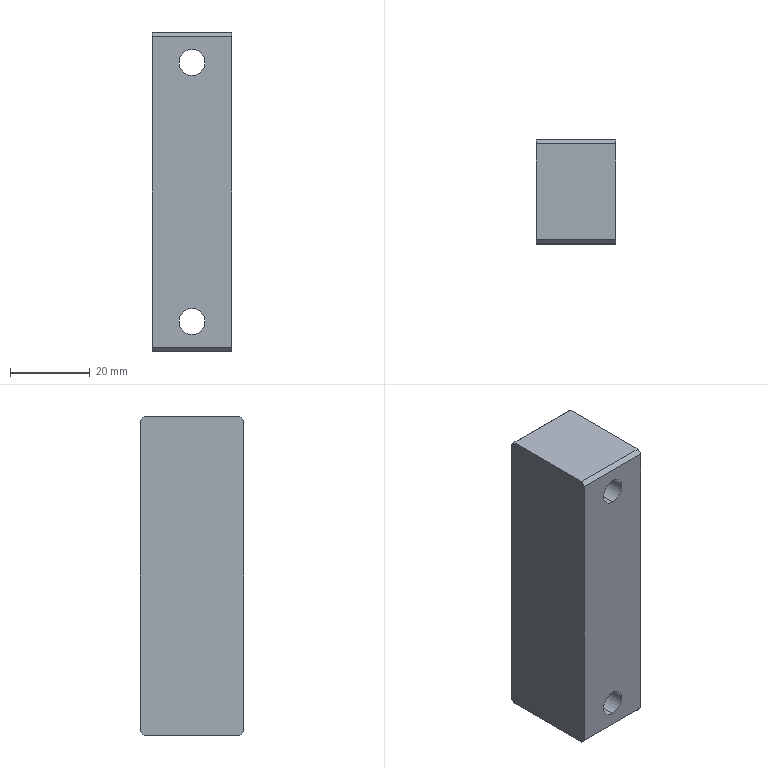Part | STEP file | Riser plate_sand-blasted, oxidised | 1 solid | 14 faces | box 20 x 26 x 80 mm | volume 39834 mm3 | plane 10 | cylinder 4 | commonest cylinder face diameters 6.5 x4
STEP:
#1=CARTESIAN_POINT('',(0.,0.,0.));
#2=DIRECTION('',(0.,0.,1.));
#3=DIRECTION('',(1.,0.,0.));
#4=AXIS2_PLACEMENT_3D('',#1,#2,#3);
#5=CARTESIAN_POINT('',(-10.,-13.65,-29.25));
#6=VERTEX_POINT('',#5);
#7=CARTESIAN_POINT('',(-10.,12.35,-29.25));
#8=VERTEX_POINT('',#7);
#9=CARTESIAN_POINT('',(-10.,97.,-29.25));
#10=DIRECTION('',(0.,1.,0.));
#11=VECTOR('',#10,1.);
#12=LINE('',#9,#11);
#13=CARTESIAN_POINT('',(-10.,97.,-32.5));
#14=DIRECTION('',(0.,1.,0.));
#15=DIRECTION('',(0.,0.,1.));
#16=AXIS2_PLACEMENT_3D('',#13,#14,#15);
#17=CYLINDRICAL_SURFACE('',#16,3.25);
#18=CARTESIAN_POINT('',(6.283,0.));
#19=DIRECTION('',(0.,1.));
#20=VECTOR('',#19,1.);
#21=LINE('',#18,#20);
#22=(GEOMETRIC_REPRESENTATION_CONTEXT(2)PARAMETRIC_REPRESENTATION_CONTEXT()REPRESENTATION_CONTEXT('',''));
#23=DEFINITIONAL_REPRESENTATION('',(#21),#22);
#24=PCURVE('',#17,#23);
#25=CARTESIAN_POINT('',(-10.,97.,-32.5));
#26=DIRECTION('',(0.,1.,0.));
#27=DIRECTION('',(0.,0.,1.));
#28=AXIS2_PLACEMENT_3D('',#25,#26,#27);
#29=CYLINDRICAL_SURFACE('',#28,3.25);
#30=CARTESIAN_POINT('',(0.,0.));
#31=DIRECTION('',(0.,1.));
#32=VECTOR('',#31,1.);
#33=LINE('',#30,#32);
#34=(GEOMETRIC_REPRESENTATION_CONTEXT(2)PARAMETRIC_REPRESENTATION_CONTEXT()REPRESENTATION_CONTEXT('',''));
#35=DEFINITIONAL_REPRESENTATION('',(#33),#34);
#36=PCURVE('',#29,#35);
#37=SURFACE_CURVE('',#12,(#24,#36),.PCURVE_S1.);
#38=EDGE_CURVE('',#6,#8,#37,.T.);
#39=ORIENTED_EDGE('',*,*,#38,.T.);
#40=CARTESIAN_POINT('',(-10.,12.35,-35.75));
#41=VERTEX_POINT('',#40);
#42=CARTESIAN_POINT('',(-10.,12.35,-32.5));
#43=DIRECTION('',(0.,-1.,0.));
#44=DIRECTION('',(0.,0.,-1.));
#45=AXIS2_PLACEMENT_3D('',#42,#43,#44);
#46=CIRCLE('',#45,3.25);
#47=CARTESIAN_POINT('',(9.425,-84.65));
#48=DIRECTION('',(-1.,0.));
#49=VECTOR('',#48,1.);
#50=LINE('',#47,#49);
#51=(GEOMETRIC_REPRESENTATION_CONTEXT(2)PARAMETRIC_REPRESENTATION_CONTEXT()REPRESENTATION_CONTEXT('',''));
#52=DEFINITIONAL_REPRESENTATION('',(#50),#51);
#53=PCURVE('',#17,#52);
#54=CARTESIAN_POINT('',(0.,12.35,-40.));
#55=DIRECTION('',(0.,-1.,0.));
#56=DIRECTION('',(0.,0.,-1.));
#57=AXIS2_PLACEMENT_3D('',#54,#55,#56);
#58=PLANE('',#57);
#59=CARTESIAN_POINT('',(-7.5,-10.));
#60=DIRECTION('',(1.,0.));
#61=AXIS2_PLACEMENT_2D('',#59,#60);
#62=CIRCLE('',#61,3.25);
#63=(GEOMETRIC_REPRESENTATION_CONTEXT(2)PARAMETRIC_REPRESENTATION_CONTEXT()REPRESENTATION_CONTEXT('',''));
#64=DEFINITIONAL_REPRESENTATION('',(#62),#63);
#65=PCURVE('',#58,#64);
#66=SURFACE_CURVE('',#46,(#53,#65),.PCURVE_S1.);
#67=EDGE_CURVE('',#8,#41,#66,.T.);
#68=ORIENTED_EDGE('',*,*,#67,.T.);
#69=CARTESIAN_POINT('',(-10.,-13.65,-35.75));
#70=VERTEX_POINT('',#69);
#71=CARTESIAN_POINT('',(-10.,97.,-35.75));
#72=DIRECTION('',(0.,1.,0.));
#73=VECTOR('',#72,1.);
#74=LINE('',#71,#73);
#75=CARTESIAN_POINT('',(3.142,0.));
#76=DIRECTION('',(0.,1.));
#77=VECTOR('',#76,1.);
#78=LINE('',#75,#77);
#79=(GEOMETRIC_REPRESENTATION_CONTEXT(2)PARAMETRIC_REPRESENTATION_CONTEXT()REPRESENTATION_CONTEXT('',''));
#80=DEFINITIONAL_REPRESENTATION('',(#78),#79);
#81=PCURVE('',#17,#80);
#82=CARTESIAN_POINT('',(3.142,0.));
#83=DIRECTION('',(0.,1.));
#84=VECTOR('',#83,1.);
#85=LINE('',#82,#84);
#86=(GEOMETRIC_REPRESENTATION_CONTEXT(2)PARAMETRIC_REPRESENTATION_CONTEXT()REPRESENTATION_CONTEXT('',''));
#87=DEFINITIONAL_REPRESENTATION('',(#85),#86);
#88=PCURVE('',#29,#87);
#89=SURFACE_CURVE('',#74,(#81,#88),.PCURVE_S1.);
#90=EDGE_CURVE('',#70,#41,#89,.T.);
#91=ORIENTED_EDGE('',*,*,#90,.F.);
#92=CARTESIAN_POINT('',(-10.,-13.65,-32.5));
#93=DIRECTION('',(0.,1.,0.));
#94=DIRECTION('',(0.,0.,1.));
#95=AXIS2_PLACEMENT_3D('',#92,#93,#94);
#96=CIRCLE('',#95,3.25);
#97=CARTESIAN_POINT('',(0.,-110.65));
#98=DIRECTION('',(1.,0.));
#99=VECTOR('',#98,1.);
#100=LINE('',#97,#99);
#101=(GEOMETRIC_REPRESENTATION_CONTEXT(2)PARAMETRIC_REPRESENTATION_CONTEXT()REPRESENTATION_CONTEXT('',''));
#102=DEFINITIONAL_REPRESENTATION('',(#100),#101);
#103=PCURVE('',#17,#102);
#104=CARTESIAN_POINT('',(0.,-13.65,40.));
#105=DIRECTION('',(0.,1.,0.));
#106=DIRECTION('',(-1.,0.,0.));
#107=AXIS2_PLACEMENT_3D('',#104,#105,#106);
#108=PLANE('',#107);
#109=CARTESIAN_POINT('',(10.,-72.5));
#110=DIRECTION('',(0.,1.));
#111=AXIS2_PLACEMENT_2D('',#109,#110);
#112=CIRCLE('',#111,3.25);
#113=(GEOMETRIC_REPRESENTATION_CONTEXT(2)PARAMETRIC_REPRESENTATION_CONTEXT()REPRESENTATION_CONTEXT('',''));
#114=DEFINITIONAL_REPRESENTATION('',(#112),#113);
#115=PCURVE('',#108,#114);
#116=SURFACE_CURVE('',#96,(#103,#115),.PCURVE_S1.);
#117=EDGE_CURVE('',#70,#6,#116,.T.);
#118=ORIENTED_EDGE('',*,*,#117,.T.);
#119=EDGE_LOOP('',(#39,#68,#91,#118));
#120=FACE_BOUND('',#119,.F.);
#121=ADVANCED_FACE('',(#120),#17,.F.);
#122=CARTESIAN_POINT('',(-10.,-13.65,35.75));
#123=VERTEX_POINT('',#122);
#124=CARTESIAN_POINT('',(-10.,12.35,35.75));
#125=VERTEX_POINT('',#124);
#126=CARTESIAN_POINT('',(-10.,97.,35.75));
#127=DIRECTION('',(0.,1.,0.));
#128=VECTOR('',#127,1.);
#129=LINE('',#126,#128);
#130=CARTESIAN_POINT('',(-10.,97.,32.5));
#131=DIRECTION('',(0.,1.,0.));
#132=DIRECTION('',(0.,0.,1.));
#133=AXIS2_PLACEMENT_3D('',#130,#131,#132);
#134=CYLINDRICAL_SURFACE('',#133,3.25);
#135=CARTESIAN_POINT('',(6.283,0.));
#136=DIRECTION('',(0.,1.));
#137=VECTOR('',#136,1.);
#138=LINE('',#135,#137);
#139=(GEOMETRIC_REPRESENTATION_CONTEXT(2)PARAMETRIC_REPRESENTATION_CONTEXT()REPRESENTATION_CONTEXT('',''));
#140=DEFINITIONAL_REPRESENTATION('',(#138),#139);
#141=PCURVE('',#134,#140);
#142=CARTESIAN_POINT('',(-10.,97.,32.5));
#143=DIRECTION('',(0.,1.,0.));
#144=DIRECTION('',(0.,0.,1.));
#145=AXIS2_PLACEMENT_3D('',#142,#143,#144);
#146=CYLINDRICAL_SURFACE('',#145,3.25);
#147=CARTESIAN_POINT('',(0.,0.));
#148=DIRECTION('',(0.,1.));
#149=VECTOR('',#148,1.);
#150=LINE('',#147,#149);
#151=(GEOMETRIC_REPRESENTATION_CONTEXT(2)PARAMETRIC_REPRESENTATION_CONTEXT()REPRESENTATION_CONTEXT('',''));
#152=DEFINITIONAL_REPRESENTATION('',(#150),#151);
#153=PCURVE('',#146,#152);
#154=SURFACE_CURVE('',#129,(#141,#153),.PCURVE_S1.);
#155=EDGE_CURVE('',#123,#125,#154,.T.);
#156=ORIENTED_EDGE('',*,*,#155,.T.);
#157=CARTESIAN_POINT('',(-10.,12.35,29.25));
#158=VERTEX_POINT('',#157);
#159=CARTESIAN_POINT('',(-10.,12.35,32.5));
#160=DIRECTION('',(0.,-1.,0.));
#161=DIRECTION('',(0.,0.,-1.));
#162=AXIS2_PLACEMENT_3D('',#159,#160,#161);
#163=CIRCLE('',#162,3.25);
#164=CARTESIAN_POINT('',(9.425,-84.65));
#165=DIRECTION('',(-1.,0.));
#166=VECTOR('',#165,1.);
#167=LINE('',#164,#166);
#168=(GEOMETRIC_REPRESENTATION_CONTEXT(2)PARAMETRIC_REPRESENTATION_CONTEXT()REPRESENTATION_CONTEXT('',''));
#169=DEFINITIONAL_REPRESENTATION('',(#167),#168);
#170=PCURVE('',#134,#169);
#171=CARTESIAN_POINT('',(-72.5,-10.));
#172=DIRECTION('',(1.,0.));
#173=AXIS2_PLACEMENT_2D('',#171,#172);
#174=CIRCLE('',#173,3.25);
#175=(GEOMETRIC_REPRESENTATION_CONTEXT(2)PARAMETRIC_REPRESENTATION_CONTEXT()REPRESENTATION_CONTEXT('',''));
#176=DEFINITIONAL_REPRESENTATION('',(#174),#175);
#177=PCURVE('',#58,#176);
#178=SURFACE_CURVE('',#163,(#170,#177),.PCURVE_S1.);
#179=EDGE_CURVE('',#125,#158,#178,.T.);
#180=ORIENTED_EDGE('',*,*,#179,.T.);
#181=CARTESIAN_POINT('',(-10.,-13.65,29.25));
#182=VERTEX_POINT('',#181);
#183=CARTESIAN_POINT('',(-10.,97.,29.25));
#184=DIRECTION('',(0.,1.,0.));
#185=VECTOR('',#184,1.);
#186=LINE('',#183,#185);
#187=CARTESIAN_POINT('',(3.142,0.));
#188=DIRECTION('',(0.,1.));
#189=VECTOR('',#188,1.);
#190=LINE('',#187,#189);
#191=(GEOMETRIC_REPRESENTATION_CONTEXT(2)PARAMETRIC_REPRESENTATION_CONTEXT()REPRESENTATION_CONTEXT('',''));
#192=DEFINITIONAL_REPRESENTATION('',(#190),#191);
#193=PCURVE('',#134,#192);
#194=CARTESIAN_POINT('',(3.142,0.));
#195=DIRECTION('',(0.,1.));
#196=VECTOR('',#195,1.);
#197=LINE('',#194,#196);
#198=(GEOMETRIC_REPRESENTATION_CONTEXT(2)PARAMETRIC_REPRESENTATION_CONTEXT()REPRESENTATION_CONTEXT('',''));
#199=DEFINITIONAL_REPRESENTATION('',(#197),#198);
#200=PCURVE('',#146,#199);
#201=SURFACE_CURVE('',#186,(#193,#200),.PCURVE_S1.);
#202=EDGE_CURVE('',#182,#158,#201,.T.);
#203=ORIENTED_EDGE('',*,*,#202,.F.);
#204=CARTESIAN_POINT('',(-10.,-13.65,32.5));
#205=DIRECTION('',(0.,1.,0.));
#206=DIRECTION('',(0.,0.,1.));
#207=AXIS2_PLACEMENT_3D('',#204,#205,#206);
#208=CIRCLE('',#207,3.25);
#209=CARTESIAN_POINT('',(0.,-110.65));
#210=DIRECTION('',(1.,0.));
#211=VECTOR('',#210,1.);
#212=LINE('',#209,#211);
#213=(GEOMETRIC_REPRESENTATION_CONTEXT(2)PARAMETRIC_REPRESENTATION_CONTEXT()REPRESENTATION_CONTEXT('',''));
#214=DEFINITIONAL_REPRESENTATION('',(#212),#213);
#215=PCURVE('',#134,#214);
#216=CARTESIAN_POINT('',(10.,-7.5));
#217=DIRECTION('',(0.,1.));
#218=AXIS2_PLACEMENT_2D('',#216,#217);
#219=CIRCLE('',#218,3.25);
#220=(GEOMETRIC_REPRESENTATION_CONTEXT(2)PARAMETRIC_REPRESENTATION_CONTEXT()REPRESENTATION_CONTEXT('',''));
#221=DEFINITIONAL_REPRESENTATION('',(#219),#220);
#222=PCURVE('',#108,#221);
#223=SURFACE_CURVE('',#208,(#215,#222),.PCURVE_S1.);
#224=EDGE_CURVE('',#182,#123,#223,.T.);
#225=ORIENTED_EDGE('',*,*,#224,.T.);
#226=EDGE_LOOP('',(#156,#180,#203,#225));
#227=FACE_BOUND('',#226,.F.);
#228=ADVANCED_FACE('',(#227),#134,.F.);
#229=CARTESIAN_POINT('',(-20.,11.35,40.));
#230=VERTEX_POINT('',#229);
#231=CARTESIAN_POINT('',(-20.,-12.65,40.));
#232=VERTEX_POINT('',#231);
#233=CARTESIAN_POINT('',(-20.,0.,40.));
#234=DIRECTION('',(0.,-1.,0.));
#235=VECTOR('',#234,1.);
#236=LINE('',#233,#235);
#237=CARTESIAN_POINT('',(0.,0.,40.));
#238=DIRECTION('',(0.,0.,-1.));
#239=DIRECTION('',(-1.,0.,0.));
#240=AXIS2_PLACEMENT_3D('',#237,#238,#239);
#241=PLANE('',#240);
#242=CARTESIAN_POINT('',(20.,0.));
#243=DIRECTION('',(0.,-1.));
#244=VECTOR('',#243,1.);
#245=LINE('',#242,#244);
#246=(GEOMETRIC_REPRESENTATION_CONTEXT(2)PARAMETRIC_REPRESENTATION_CONTEXT()REPRESENTATION_CONTEXT('',''));
#247=DEFINITIONAL_REPRESENTATION('',(#245),#246);
#248=PCURVE('',#241,#247);
#249=CARTESIAN_POINT('',(-20.,0.,40.));
#250=DIRECTION('',(1.,0.,0.));
#251=DIRECTION('',(0.,0.,-1.));
#252=AXIS2_PLACEMENT_3D('',#249,#250,#251);
#253=PLANE('',#252);
#254=CARTESIAN_POINT('',(0.,0.));
#255=DIRECTION('',(0.,-1.));
#256=VECTOR('',#255,1.);
#257=LINE('',#254,#256);
#258=(GEOMETRIC_REPRESENTATION_CONTEXT(2)PARAMETRIC_REPRESENTATION_CONTEXT()REPRESENTATION_CONTEXT('',''));
#259=DEFINITIONAL_REPRESENTATION('',(#257),#258);
#260=PCURVE('',#253,#259);
#261=SURFACE_CURVE('',#236,(#248,#260),.PCURVE_S1.);
#262=EDGE_CURVE('',#230,#232,#261,.T.);
#263=ORIENTED_EDGE('',*,*,#262,.T.);
#264=CARTESIAN_POINT('',(0.,-12.65,40.));
#265=VERTEX_POINT('',#264);
#266=CARTESIAN_POINT('',(0.,-12.65,40.));
#267=DIRECTION('',(1.,0.,0.));
#268=VECTOR('',#267,1.);
#269=LINE('',#266,#268);
#270=CARTESIAN_POINT('',(0.,-12.65));
#271=DIRECTION('',(-1.,0.));
#272=VECTOR('',#271,1.);
#273=LINE('',#270,#272);
#274=(GEOMETRIC_REPRESENTATION_CONTEXT(2)PARAMETRIC_REPRESENTATION_CONTEXT()REPRESENTATION_CONTEXT('',''));
#275=DEFINITIONAL_REPRESENTATION('',(#273),#274);
#276=PCURVE('',#241,#275);
#277=CARTESIAN_POINT('',(0.,-12.65,40.));
#278=DIRECTION('',(0.,0.7071,-0.7071));
#279=DIRECTION('',(1.,0.,0.));
#280=AXIS2_PLACEMENT_3D('',#277,#278,#279);
#281=PLANE('',#280);
#282=CARTESIAN_POINT('',(0.,0.));
#283=DIRECTION('',(1.,0.));
#284=VECTOR('',#283,1.);
#285=LINE('',#282,#284);
#286=(GEOMETRIC_REPRESENTATION_CONTEXT(2)PARAMETRIC_REPRESENTATION_CONTEXT()REPRESENTATION_CONTEXT('',''));
#287=DEFINITIONAL_REPRESENTATION('',(#285),#286);
#288=PCURVE('',#281,#287);
#289=SURFACE_CURVE('',#269,(#276,#288),.PCURVE_S1.);
#290=EDGE_CURVE('',#232,#265,#289,.T.);
#291=ORIENTED_EDGE('',*,*,#290,.T.);
#292=CARTESIAN_POINT('',(0.,11.35,40.));
#293=VERTEX_POINT('',#292);
#294=CARTESIAN_POINT('',(0.,97.,40.));
#295=DIRECTION('',(0.,1.,0.));
#296=VECTOR('',#295,1.);
#297=LINE('',#294,#296);
#298=CARTESIAN_POINT('',(0.,97.));
#299=DIRECTION('',(0.,1.));
#300=VECTOR('',#299,1.);
#301=LINE('',#298,#300);
#302=(GEOMETRIC_REPRESENTATION_CONTEXT(2)PARAMETRIC_REPRESENTATION_CONTEXT()REPRESENTATION_CONTEXT('',''));
#303=DEFINITIONAL_REPRESENTATION('',(#301),#302);
#304=PCURVE('',#241,#303);
#305=CARTESIAN_POINT('',(0.,97.,40.));
#306=DIRECTION('',(-1.,0.,0.));
#307=DIRECTION('',(0.,-1.,0.));
#308=AXIS2_PLACEMENT_3D('',#305,#306,#307);
#309=PLANE('',#308);
#310=CARTESIAN_POINT('',(0.,0.));
#311=DIRECTION('',(-1.,0.));
#312=VECTOR('',#311,1.);
#313=LINE('',#310,#312);
#314=(GEOMETRIC_REPRESENTATION_CONTEXT(2)PARAMETRIC_REPRESENTATION_CONTEXT()REPRESENTATION_CONTEXT('',''));
#315=DEFINITIONAL_REPRESENTATION('',(#313),#314);
#316=PCURVE('',#309,#315);
#317=SURFACE_CURVE('',#297,(#304,#316),.PCURVE_S1.);
#318=EDGE_CURVE('',#265,#293,#317,.T.);
#319=ORIENTED_EDGE('',*,*,#318,.T.);
#320=CARTESIAN_POINT('',(0.,11.35,40.));
#321=DIRECTION('',(-1.,0.,0.));
#322=VECTOR('',#321,1.);
#323=LINE('',#320,#322);
#324=CARTESIAN_POINT('',(0.,11.35));
#325=DIRECTION('',(1.,0.));
#326=VECTOR('',#325,1.);
#327=LINE('',#324,#326);
#328=(GEOMETRIC_REPRESENTATION_CONTEXT(2)PARAMETRIC_REPRESENTATION_CONTEXT()REPRESENTATION_CONTEXT('',''));
#329=DEFINITIONAL_REPRESENTATION('',(#327),#328);
#330=PCURVE('',#241,#329);
#331=CARTESIAN_POINT('',(0.,11.35,40.));
#332=DIRECTION('',(0.,-0.7071,-0.7071));
#333=DIRECTION('',(-1.,0.,0.));
#334=AXIS2_PLACEMENT_3D('',#331,#332,#333);
#335=PLANE('',#334);
#336=CARTESIAN_POINT('',(0.,0.));
#337=DIRECTION('',(1.,0.));
#338=VECTOR('',#337,1.);
#339=LINE('',#336,#338);
#340=(GEOMETRIC_REPRESENTATION_CONTEXT(2)PARAMETRIC_REPRESENTATION_CONTEXT()REPRESENTATION_CONTEXT('',''));
#341=DEFINITIONAL_REPRESENTATION('',(#339),#340);
#342=PCURVE('',#335,#341);
#343=SURFACE_CURVE('',#323,(#330,#342),.PCURVE_S1.);
#344=EDGE_CURVE('',#293,#230,#343,.T.);
#345=ORIENTED_EDGE('',*,*,#344,.T.);
#346=EDGE_LOOP('',(#263,#291,#319,#345));
#347=FACE_BOUND('',#346,.T.);
#348=ADVANCED_FACE('',(#347),#241,.F.);
#349=CARTESIAN_POINT('',(0.,11.35,-40.));
#350=VERTEX_POINT('',#349);
#351=CARTESIAN_POINT('',(0.,12.35,-39.));
#352=VERTEX_POINT('',#351);
#353=CARTESIAN_POINT('',(0.,12.35,-39.));
#354=DIRECTION('',(0.,0.7071,0.7071));
#355=VECTOR('',#354,1.);
#356=LINE('',#353,#355);
#357=CARTESIAN_POINT('',(84.65,-79.));
#358=DIRECTION('',(-0.7071,0.7071));
#359=VECTOR('',#358,1.);
#360=LINE('',#357,#359);
#361=(GEOMETRIC_REPRESENTATION_CONTEXT(2)PARAMETRIC_REPRESENTATION_CONTEXT()REPRESENTATION_CONTEXT('',''));
#362=DEFINITIONAL_REPRESENTATION('',(#360),#361);
#363=PCURVE('',#309,#362);
#364=CARTESIAN_POINT('',(0.,12.35,-39.));
#365=DIRECTION('',(0.,0.7071,-0.7071));
#366=DIRECTION('',(1.,0.,0.));
#367=AXIS2_PLACEMENT_3D('',#364,#365,#366);
#368=PLANE('',#367);
#369=CARTESIAN_POINT('',(0.,0.));
#370=DIRECTION('',(0.,-1.));
#371=VECTOR('',#370,1.);
#372=LINE('',#369,#371);
#373=(GEOMETRIC_REPRESENTATION_CONTEXT(2)PARAMETRIC_REPRESENTATION_CONTEXT()REPRESENTATION_CONTEXT('',''));
#374=DEFINITIONAL_REPRESENTATION('',(#372),#373);
#375=PCURVE('',#368,#374);
#376=SURFACE_CURVE('',#356,(#363,#375),.PCURVE_S1.);
#377=EDGE_CURVE('',#350,#352,#376,.T.);
#378=ORIENTED_EDGE('',*,*,#377,.T.);
#379=CARTESIAN_POINT('',(0.,12.35,39.));
#380=VERTEX_POINT('',#379);
#381=CARTESIAN_POINT('',(0.,12.35,40.));
#382=DIRECTION('',(0.,0.,1.));
#383=VECTOR('',#382,1.);
#384=LINE('',#381,#383);
#385=CARTESIAN_POINT('',(84.65,0.));
#386=DIRECTION('',(0.,1.));
#387=VECTOR('',#386,1.);
#388=LINE('',#385,#387);
#389=(GEOMETRIC_REPRESENTATION_CONTEXT(2)PARAMETRIC_REPRESENTATION_CONTEXT()REPRESENTATION_CONTEXT('',''));
#390=DEFINITIONAL_REPRESENTATION('',(#388),#389);
#391=PCURVE('',#309,#390);
#392=CARTESIAN_POINT('',(-80.,0.));
#393=DIRECTION('',(-1.,0.));
#394=VECTOR('',#393,1.);
#395=LINE('',#392,#394);
#396=(GEOMETRIC_REPRESENTATION_CONTEXT(2)PARAMETRIC_REPRESENTATION_CONTEXT()REPRESENTATION_CONTEXT('',''));
#397=DEFINITIONAL_REPRESENTATION('',(#395),#396);
#398=PCURVE('',#58,#397);
#399=SURFACE_CURVE('',#384,(#391,#398),.PCURVE_S1.);
#400=EDGE_CURVE('',#352,#380,#399,.T.);
#401=ORIENTED_EDGE('',*,*,#400,.T.);
#402=CARTESIAN_POINT('',(0.,11.35,40.));
#403=DIRECTION('',(0.,-0.7071,0.7071));
#404=VECTOR('',#403,1.);
#405=LINE('',#402,#404);
#406=CARTESIAN_POINT('',(85.65,0.));
#407=DIRECTION('',(0.7071,0.7071));
#408=VECTOR('',#407,1.);
#409=LINE('',#406,#408);
#410=(GEOMETRIC_REPRESENTATION_CONTEXT(2)PARAMETRIC_REPRESENTATION_CONTEXT()REPRESENTATION_CONTEXT('',''));
#411=DEFINITIONAL_REPRESENTATION('',(#409),#410);
#412=PCURVE('',#309,#411);
#413=CARTESIAN_POINT('',(0.,0.));
#414=DIRECTION('',(0.,-1.));
#415=VECTOR('',#414,1.);
#416=LINE('',#413,#415);
#417=(GEOMETRIC_REPRESENTATION_CONTEXT(2)PARAMETRIC_REPRESENTATION_CONTEXT()REPRESENTATION_CONTEXT('',''));
#418=DEFINITIONAL_REPRESENTATION('',(#416),#417);
#419=PCURVE('',#335,#418);
#420=SURFACE_CURVE('',#405,(#412,#419),.PCURVE_S1.);
#421=EDGE_CURVE('',#380,#293,#420,.T.);
#422=ORIENTED_EDGE('',*,*,#421,.T.);
#423=ORIENTED_EDGE('',*,*,#318,.F.);
#424=CARTESIAN_POINT('',(0.,-13.65,39.));
#425=VERTEX_POINT('',#424);
#426=CARTESIAN_POINT('',(0.,-12.65,40.));
#427=DIRECTION('',(0.,-0.7071,-0.7071));
#428=VECTOR('',#427,1.);
#429=LINE('',#426,#428);
#430=CARTESIAN_POINT('',(109.65,0.));
#431=DIRECTION('',(0.7071,-0.7071));
#432=VECTOR('',#431,1.);
#433=LINE('',#430,#432);
#434=(GEOMETRIC_REPRESENTATION_CONTEXT(2)PARAMETRIC_REPRESENTATION_CONTEXT()REPRESENTATION_CONTEXT('',''));
#435=DEFINITIONAL_REPRESENTATION('',(#433),#434);
#436=PCURVE('',#309,#435);
#437=CARTESIAN_POINT('',(0.,0.));
#438=DIRECTION('',(0.,1.));
#439=VECTOR('',#438,1.);
#440=LINE('',#437,#439);
#441=(GEOMETRIC_REPRESENTATION_CONTEXT(2)PARAMETRIC_REPRESENTATION_CONTEXT()REPRESENTATION_CONTEXT('',''));
#442=DEFINITIONAL_REPRESENTATION('',(#440),#441);
#443=PCURVE('',#281,#442);
#444=SURFACE_CURVE('',#429,(#436,#443),.PCURVE_S1.);
#445=EDGE_CURVE('',#265,#425,#444,.T.);
#446=ORIENTED_EDGE('',*,*,#445,.T.);
#447=CARTESIAN_POINT('',(0.,-13.65,-39.));
#448=VERTEX_POINT('',#447);
#449=CARTESIAN_POINT('',(0.,-13.65,40.));
#450=DIRECTION('',(0.,0.,-1.));
#451=VECTOR('',#450,1.);
#452=LINE('',#449,#451);
#453=CARTESIAN_POINT('',(110.65,0.));
#454=DIRECTION('',(0.,-1.));
#455=VECTOR('',#454,1.);
#456=LINE('',#453,#455);
#457=(GEOMETRIC_REPRESENTATION_CONTEXT(2)PARAMETRIC_REPRESENTATION_CONTEXT()REPRESENTATION_CONTEXT('',''));
#458=DEFINITIONAL_REPRESENTATION('',(#456),#457);
#459=PCURVE('',#309,#458);
#460=CARTESIAN_POINT('',(0.,0.));
#461=DIRECTION('',(0.,-1.));
#462=VECTOR('',#461,1.);
#463=LINE('',#460,#462);
#464=(GEOMETRIC_REPRESENTATION_CONTEXT(2)PARAMETRIC_REPRESENTATION_CONTEXT()REPRESENTATION_CONTEXT('',''));
#465=DEFINITIONAL_REPRESENTATION('',(#463),#464);
#466=PCURVE('',#108,#465);
#467=SURFACE_CURVE('',#452,(#459,#466),.PCURVE_S1.);
#468=EDGE_CURVE('',#425,#448,#467,.T.);
#469=ORIENTED_EDGE('',*,*,#468,.T.);
#470=CARTESIAN_POINT('',(0.,-12.65,-40.));
#471=VERTEX_POINT('',#470);
#472=CARTESIAN_POINT('',(0.,-13.65,-39.));
#473=DIRECTION('',(0.,0.7071,-0.7071));
#474=VECTOR('',#473,1.);
#475=LINE('',#472,#474);
#476=CARTESIAN_POINT('',(110.65,-79.));
#477=DIRECTION('',(-0.7071,-0.7071));
#478=VECTOR('',#477,1.);
#479=LINE('',#476,#478);
#480=(GEOMETRIC_REPRESENTATION_CONTEXT(2)PARAMETRIC_REPRESENTATION_CONTEXT()REPRESENTATION_CONTEXT('',''));
#481=DEFINITIONAL_REPRESENTATION('',(#479),#480);
#482=PCURVE('',#309,#481);
#483=CARTESIAN_POINT('',(0.,-13.65,-39.));
#484=DIRECTION('',(0.,-0.7071,-0.7071));
#485=DIRECTION('',(-1.,0.,0.));
#486=AXIS2_PLACEMENT_3D('',#483,#484,#485);
#487=PLANE('',#486);
#488=CARTESIAN_POINT('',(0.,0.));
#489=DIRECTION('',(0.,1.));
#490=VECTOR('',#489,1.);
#491=LINE('',#488,#490);
#492=(GEOMETRIC_REPRESENTATION_CONTEXT(2)PARAMETRIC_REPRESENTATION_CONTEXT()REPRESENTATION_CONTEXT('',''));
#493=DEFINITIONAL_REPRESENTATION('',(#491),#492);
#494=PCURVE('',#487,#493);
#495=SURFACE_CURVE('',#475,(#482,#494),.PCURVE_S1.);
#496=EDGE_CURVE('',#448,#471,#495,.T.);
#497=ORIENTED_EDGE('',*,*,#496,.T.);
#498=CARTESIAN_POINT('',(0.,97.,-40.));
#499=DIRECTION('',(0.,1.,0.));
#500=VECTOR('',#499,1.);
#501=LINE('',#498,#500);
#502=CARTESIAN_POINT('',(0.,-80.));
#503=DIRECTION('',(-1.,0.));
#504=VECTOR('',#503,1.);
#505=LINE('',#502,#504);
#506=(GEOMETRIC_REPRESENTATION_CONTEXT(2)PARAMETRIC_REPRESENTATION_CONTEXT()REPRESENTATION_CONTEXT('',''));
#507=DEFINITIONAL_REPRESENTATION('',(#505),#506);
#508=PCURVE('',#309,#507);
#509=CARTESIAN_POINT('',(0.,0.,-40.));
#510=DIRECTION('',(0.,0.,-1.));
#511=DIRECTION('',(-1.,0.,0.));
#512=AXIS2_PLACEMENT_3D('',#509,#510,#511);
#513=PLANE('',#512);
#514=CARTESIAN_POINT('',(0.,97.));
#515=DIRECTION('',(0.,1.));
#516=VECTOR('',#515,1.);
#517=LINE('',#514,#516);
#518=(GEOMETRIC_REPRESENTATION_CONTEXT(2)PARAMETRIC_REPRESENTATION_CONTEXT()REPRESENTATION_CONTEXT('',''));
#519=DEFINITIONAL_REPRESENTATION('',(#517),#518);
#520=PCURVE('',#513,#519);
#521=SURFACE_CURVE('',#501,(#508,#520),.PCURVE_S1.);
#522=EDGE_CURVE('',#471,#350,#521,.T.);
#523=ORIENTED_EDGE('',*,*,#522,.T.);
#524=EDGE_LOOP('',(#378,#401,#422,#423,#446,#469,#497,#523));
#525=FACE_BOUND('',#524,.T.);
#526=ADVANCED_FACE('',(#525),#309,.F.);
#527=CARTESIAN_POINT('',(-20.,12.35,-39.));
#528=VERTEX_POINT('',#527);
#529=CARTESIAN_POINT('',(-20.,12.35,39.));
#530=VERTEX_POINT('',#529);
#531=CARTESIAN_POINT('',(-20.,12.35,40.));
#532=DIRECTION('',(0.,0.,1.));
#533=VECTOR('',#532,1.);
#534=LINE('',#531,#533);
#535=CARTESIAN_POINT('',(0.,12.35));
#536=DIRECTION('',(-1.,0.));
#537=VECTOR('',#536,1.);
#538=LINE('',#535,#537);
#539=(GEOMETRIC_REPRESENTATION_CONTEXT(2)PARAMETRIC_REPRESENTATION_CONTEXT()REPRESENTATION_CONTEXT('',''));
#540=DEFINITIONAL_REPRESENTATION('',(#538),#539);
#541=PCURVE('',#253,#540);
#542=CARTESIAN_POINT('',(-80.,-20.));
#543=DIRECTION('',(-1.,0.));
#544=VECTOR('',#543,1.);
#545=LINE('',#542,#544);
#546=(GEOMETRIC_REPRESENTATION_CONTEXT(2)PARAMETRIC_REPRESENTATION_CONTEXT()REPRESENTATION_CONTEXT('',''));
#547=DEFINITIONAL_REPRESENTATION('',(#545),#546);
#548=PCURVE('',#58,#547);
#549=SURFACE_CURVE('',#534,(#541,#548),.PCURVE_S1.);
#550=EDGE_CURVE('',#528,#530,#549,.T.);
#551=ORIENTED_EDGE('',*,*,#550,.F.);
#552=CARTESIAN_POINT('',(-20.,11.35,-40.));
#553=VERTEX_POINT('',#552);
#554=CARTESIAN_POINT('',(-20.,12.35,-39.));
#555=DIRECTION('',(0.,-0.7071,-0.7071));
#556=VECTOR('',#555,1.);
#557=LINE('',#554,#556);
#558=CARTESIAN_POINT('',(79.,12.35));
#559=DIRECTION('',(0.7071,-0.7071));
#560=VECTOR('',#559,1.);
#561=LINE('',#558,#560);
#562=(GEOMETRIC_REPRESENTATION_CONTEXT(2)PARAMETRIC_REPRESENTATION_CONTEXT()REPRESENTATION_CONTEXT('',''));
#563=DEFINITIONAL_REPRESENTATION('',(#561),#562);
#564=PCURVE('',#253,#563);
#565=CARTESIAN_POINT('',(-20.,0.));
#566=DIRECTION('',(0.,1.));
#567=VECTOR('',#566,1.);
#568=LINE('',#565,#567);
#569=(GEOMETRIC_REPRESENTATION_CONTEXT(2)PARAMETRIC_REPRESENTATION_CONTEXT()REPRESENTATION_CONTEXT('',''));
#570=DEFINITIONAL_REPRESENTATION('',(#568),#569);
#571=PCURVE('',#368,#570);
#572=SURFACE_CURVE('',#557,(#564,#571),.PCURVE_S1.);
#573=EDGE_CURVE('',#528,#553,#572,.T.);
#574=ORIENTED_EDGE('',*,*,#573,.T.);
#575=CARTESIAN_POINT('',(-20.,-12.65,-40.));
#576=VERTEX_POINT('',#575);
#577=CARTESIAN_POINT('',(-20.,0.,-40.));
#578=DIRECTION('',(0.,-1.,0.));
#579=VECTOR('',#578,1.);
#580=LINE('',#577,#579);
#581=CARTESIAN_POINT('',(80.,0.));
#582=DIRECTION('',(0.,-1.));
#583=VECTOR('',#582,1.);
#584=LINE('',#581,#583);
#585=(GEOMETRIC_REPRESENTATION_CONTEXT(2)PARAMETRIC_REPRESENTATION_CONTEXT()REPRESENTATION_CONTEXT('',''));
#586=DEFINITIONAL_REPRESENTATION('',(#584),#585);
#587=PCURVE('',#253,#586);
#588=CARTESIAN_POINT('',(20.,0.));
#589=DIRECTION('',(0.,-1.));
#590=VECTOR('',#589,1.);
#591=LINE('',#588,#590);
#592=(GEOMETRIC_REPRESENTATION_CONTEXT(2)PARAMETRIC_REPRESENTATION_CONTEXT()REPRESENTATION_CONTEXT('',''));
#593=DEFINITIONAL_REPRESENTATION('',(#591),#592);
#594=PCURVE('',#513,#593);
#595=SURFACE_CURVE('',#580,(#587,#594),.PCURVE_S1.);
#596=EDGE_CURVE('',#553,#576,#595,.T.);
#597=ORIENTED_EDGE('',*,*,#596,.T.);
#598=CARTESIAN_POINT('',(-20.,-13.65,-39.));
#599=VERTEX_POINT('',#598);
#600=CARTESIAN_POINT('',(-20.,-13.65,-39.));
#601=DIRECTION('',(0.,-0.7071,0.7071));
#602=VECTOR('',#601,1.);
#603=LINE('',#600,#602);
#604=CARTESIAN_POINT('',(79.,-13.65));
#605=DIRECTION('',(-0.7071,-0.7071));
#606=VECTOR('',#605,1.);
#607=LINE('',#604,#606);
#608=(GEOMETRIC_REPRESENTATION_CONTEXT(2)PARAMETRIC_REPRESENTATION_CONTEXT()REPRESENTATION_CONTEXT('',''));
#609=DEFINITIONAL_REPRESENTATION('',(#607),#608);
#610=PCURVE('',#253,#609);
#611=CARTESIAN_POINT('',(20.,0.));
#612=DIRECTION('',(0.,-1.));
#613=VECTOR('',#612,1.);
#614=LINE('',#611,#613);
#615=(GEOMETRIC_REPRESENTATION_CONTEXT(2)PARAMETRIC_REPRESENTATION_CONTEXT()REPRESENTATION_CONTEXT('',''));
#616=DEFINITIONAL_REPRESENTATION('',(#614),#615);
#617=PCURVE('',#487,#616);
#618=SURFACE_CURVE('',#603,(#610,#617),.PCURVE_S1.);
#619=EDGE_CURVE('',#576,#599,#618,.T.);
#620=ORIENTED_EDGE('',*,*,#619,.T.);
#621=CARTESIAN_POINT('',(-20.,-13.65,39.));
#622=VERTEX_POINT('',#621);
#623=CARTESIAN_POINT('',(-20.,-13.65,40.));
#624=DIRECTION('',(0.,0.,-1.));
#625=VECTOR('',#624,1.);
#626=LINE('',#623,#625);
#627=CARTESIAN_POINT('',(0.,-13.65));
#628=DIRECTION('',(1.,0.));
#629=VECTOR('',#628,1.);
#630=LINE('',#627,#629);
#631=(GEOMETRIC_REPRESENTATION_CONTEXT(2)PARAMETRIC_REPRESENTATION_CONTEXT()REPRESENTATION_CONTEXT('',''));
#632=DEFINITIONAL_REPRESENTATION('',(#630),#631);
#633=PCURVE('',#253,#632);
#634=CARTESIAN_POINT('',(20.,0.));
#635=DIRECTION('',(0.,-1.));
#636=VECTOR('',#635,1.);
#637=LINE('',#634,#636);
#638=(GEOMETRIC_REPRESENTATION_CONTEXT(2)PARAMETRIC_REPRESENTATION_CONTEXT()REPRESENTATION_CONTEXT('',''));
#639=DEFINITIONAL_REPRESENTATION('',(#637),#638);
#640=PCURVE('',#108,#639);
#641=SURFACE_CURVE('',#626,(#633,#640),.PCURVE_S1.);
#642=EDGE_CURVE('',#622,#599,#641,.T.);
#643=ORIENTED_EDGE('',*,*,#642,.F.);
#644=CARTESIAN_POINT('',(-20.,-12.65,40.));
#645=DIRECTION('',(0.,0.7071,0.7071));
#646=VECTOR('',#645,1.);
#647=LINE('',#644,#646);
#648=CARTESIAN_POINT('',(0.,-12.65));
#649=DIRECTION('',(-0.7071,0.7071));
#650=VECTOR('',#649,1.);
#651=LINE('',#648,#650);
#652=(GEOMETRIC_REPRESENTATION_CONTEXT(2)PARAMETRIC_REPRESENTATION_CONTEXT()REPRESENTATION_CONTEXT('',''));
#653=DEFINITIONAL_REPRESENTATION('',(#651),#652);
#654=PCURVE('',#253,#653);
#655=CARTESIAN_POINT('',(-20.,0.));
#656=DIRECTION('',(0.,-1.));
#657=VECTOR('',#656,1.);
#658=LINE('',#655,#657);
#659=(GEOMETRIC_REPRESENTATION_CONTEXT(2)PARAMETRIC_REPRESENTATION_CONTEXT()REPRESENTATION_CONTEXT('',''));
#660=DEFINITIONAL_REPRESENTATION('',(#658),#659);
#661=PCURVE('',#281,#660);
#662=SURFACE_CURVE('',#647,(#654,#661),.PCURVE_S1.);
#663=EDGE_CURVE('',#622,#232,#662,.T.);
#664=ORIENTED_EDGE('',*,*,#663,.T.);
#665=ORIENTED_EDGE('',*,*,#262,.F.);
#666=CARTESIAN_POINT('',(-20.,11.35,40.));
#667=DIRECTION('',(0.,0.7071,-0.7071));
#668=VECTOR('',#667,1.);
#669=LINE('',#666,#668);
#670=CARTESIAN_POINT('',(0.,11.35));
#671=DIRECTION('',(0.7071,0.7071));
#672=VECTOR('',#671,1.);
#673=LINE('',#670,#672);
#674=(GEOMETRIC_REPRESENTATION_CONTEXT(2)PARAMETRIC_REPRESENTATION_CONTEXT()REPRESENTATION_CONTEXT('',''));
#675=DEFINITIONAL_REPRESENTATION('',(#673),#674);
#676=PCURVE('',#253,#675);
#677=CARTESIAN_POINT('',(20.,0.));
#678=DIRECTION('',(0.,1.));
#679=VECTOR('',#678,1.);
#680=LINE('',#677,#679);
#681=(GEOMETRIC_REPRESENTATION_CONTEXT(2)PARAMETRIC_REPRESENTATION_CONTEXT()REPRESENTATION_CONTEXT('',''));
#682=DEFINITIONAL_REPRESENTATION('',(#680),#681);
#683=PCURVE('',#335,#682);
#684=SURFACE_CURVE('',#669,(#676,#683),.PCURVE_S1.);
#685=EDGE_CURVE('',#230,#530,#684,.T.);
#686=ORIENTED_EDGE('',*,*,#685,.T.);
#687=EDGE_LOOP('',(#551,#574,#597,#620,#643,#664,#665,#686));
#688=FACE_BOUND('',#687,.T.);
#689=ADVANCED_FACE('',(#688),#253,.F.);
#690=CARTESIAN_POINT('',(-10.,-13.65,-32.5));
#691=DIRECTION('',(0.,1.,0.));
#692=DIRECTION('',(0.,0.,1.));
#693=AXIS2_PLACEMENT_3D('',#690,#691,#692);
#694=CIRCLE('',#693,3.25);
#695=CARTESIAN_POINT('',(10.,-72.5));
#696=DIRECTION('',(0.,1.));
#697=AXIS2_PLACEMENT_2D('',#695,#696);
#698=CIRCLE('',#697,3.25);
#699=(GEOMETRIC_REPRESENTATION_CONTEXT(2)PARAMETRIC_REPRESENTATION_CONTEXT()REPRESENTATION_CONTEXT('',''));
#700=DEFINITIONAL_REPRESENTATION('',(#698),#699);
#701=PCURVE('',#108,#700);
#702=CARTESIAN_POINT('',(0.,-110.65));
#703=DIRECTION('',(1.,0.));
#704=VECTOR('',#703,1.);
#705=LINE('',#702,#704);
#706=(GEOMETRIC_REPRESENTATION_CONTEXT(2)PARAMETRIC_REPRESENTATION_CONTEXT()REPRESENTATION_CONTEXT('',''));
#707=DEFINITIONAL_REPRESENTATION('',(#705),#706);
#708=PCURVE('',#29,#707);
#709=SURFACE_CURVE('',#694,(#701,#708),.PCURVE_S1.);
#710=EDGE_CURVE('',#6,#70,#709,.T.);
#711=ORIENTED_EDGE('',*,*,#710,.T.);
#712=ORIENTED_EDGE('',*,*,#117,.T.);
#713=EDGE_LOOP('',(#711,#712));
#714=FACE_BOUND('',#713,.T.);
#715=CARTESIAN_POINT('',(-10.,-13.65,32.5));
#716=DIRECTION('',(0.,1.,0.));
#717=DIRECTION('',(0.,0.,1.));
#718=AXIS2_PLACEMENT_3D('',#715,#716,#717);
#719=CIRCLE('',#718,3.25);
#720=CARTESIAN_POINT('',(10.,-7.5));
#721=DIRECTION('',(0.,1.));
#722=AXIS2_PLACEMENT_2D('',#720,#721);
#723=CIRCLE('',#722,3.25);
#724=(GEOMETRIC_REPRESENTATION_CONTEXT(2)PARAMETRIC_REPRESENTATION_CONTEXT()REPRESENTATION_CONTEXT('',''));
#725=DEFINITIONAL_REPRESENTATION('',(#723),#724);
#726=PCURVE('',#108,#725);
#727=CARTESIAN_POINT('',(0.,-110.65));
#728=DIRECTION('',(1.,0.));
#729=VECTOR('',#728,1.);
#730=LINE('',#727,#729);
#731=(GEOMETRIC_REPRESENTATION_CONTEXT(2)PARAMETRIC_REPRESENTATION_CONTEXT()REPRESENTATION_CONTEXT('',''));
#732=DEFINITIONAL_REPRESENTATION('',(#730),#731);
#733=PCURVE('',#146,#732);
#734=SURFACE_CURVE('',#719,(#726,#733),.PCURVE_S1.);
#735=EDGE_CURVE('',#123,#182,#734,.T.);
#736=ORIENTED_EDGE('',*,*,#735,.T.);
#737=ORIENTED_EDGE('',*,*,#224,.T.);
#738=EDGE_LOOP('',(#736,#737));
#739=FACE_BOUND('',#738,.T.);
#740=ORIENTED_EDGE('',*,*,#468,.F.);
#741=CARTESIAN_POINT('',(0.,-13.65,39.));
#742=DIRECTION('',(-1.,0.,0.));
#743=VECTOR('',#742,1.);
#744=LINE('',#741,#743);
#745=CARTESIAN_POINT('',(0.,-1.));
#746=DIRECTION('',(1.,0.));
#747=VECTOR('',#746,1.);
#748=LINE('',#745,#747);
#749=(GEOMETRIC_REPRESENTATION_CONTEXT(2)PARAMETRIC_REPRESENTATION_CONTEXT()REPRESENTATION_CONTEXT('',''));
#750=DEFINITIONAL_REPRESENTATION('',(#748),#749);
#751=PCURVE('',#108,#750);
#752=CARTESIAN_POINT('',(0.,1.414));
#753=DIRECTION('',(-1.,0.));
#754=VECTOR('',#753,1.);
#755=LINE('',#752,#754);
#756=(GEOMETRIC_REPRESENTATION_CONTEXT(2)PARAMETRIC_REPRESENTATION_CONTEXT()REPRESENTATION_CONTEXT('',''));
#757=DEFINITIONAL_REPRESENTATION('',(#755),#756);
#758=PCURVE('',#281,#757);
#759=SURFACE_CURVE('',#744,(#751,#758),.PCURVE_S1.);
#760=EDGE_CURVE('',#425,#622,#759,.T.);
#761=ORIENTED_EDGE('',*,*,#760,.T.);
#762=ORIENTED_EDGE('',*,*,#642,.T.);
#763=CARTESIAN_POINT('',(0.,-13.65,-39.));
#764=DIRECTION('',(1.,0.,0.));
#765=VECTOR('',#764,1.);
#766=LINE('',#763,#765);
#767=CARTESIAN_POINT('',(0.,-79.));
#768=DIRECTION('',(-1.,0.));
#769=VECTOR('',#768,1.);
#770=LINE('',#767,#769);
#771=(GEOMETRIC_REPRESENTATION_CONTEXT(2)PARAMETRIC_REPRESENTATION_CONTEXT()REPRESENTATION_CONTEXT('',''));
#772=DEFINITIONAL_REPRESENTATION('',(#770),#771);
#773=PCURVE('',#108,#772);
#774=CARTESIAN_POINT('',(0.,0.));
#775=DIRECTION('',(-1.,0.));
#776=VECTOR('',#775,1.);
#777=LINE('',#774,#776);
#778=(GEOMETRIC_REPRESENTATION_CONTEXT(2)PARAMETRIC_REPRESENTATION_CONTEXT()REPRESENTATION_CONTEXT('',''));
#779=DEFINITIONAL_REPRESENTATION('',(#777),#778);
#780=PCURVE('',#487,#779);
#781=SURFACE_CURVE('',#766,(#773,#780),.PCURVE_S1.);
#782=EDGE_CURVE('',#599,#448,#781,.T.);
#783=ORIENTED_EDGE('',*,*,#782,.T.);
#784=EDGE_LOOP('',(#740,#761,#762,#783));
#785=FACE_BOUND('',#784,.T.);
#786=ADVANCED_FACE('',(#714,#739,#785),#108,.F.);
#787=ORIENTED_EDGE('',*,*,#522,.F.);
#788=CARTESIAN_POINT('',(-20.,-12.65,-40.));
#789=DIRECTION('',(-1.,0.,0.));
#790=VECTOR('',#789,1.);
#791=LINE('',#788,#790);
#792=CARTESIAN_POINT('',(20.,-12.65));
#793=DIRECTION('',(1.,0.));
#794=VECTOR('',#793,1.);
#795=LINE('',#792,#794);
#796=(GEOMETRIC_REPRESENTATION_CONTEXT(2)PARAMETRIC_REPRESENTATION_CONTEXT()REPRESENTATION_CONTEXT('',''));
#797=DEFINITIONAL_REPRESENTATION('',(#795),#796);
#798=PCURVE('',#513,#797);
#799=CARTESIAN_POINT('',(20.,1.414));
#800=DIRECTION('',(1.,0.));
#801=VECTOR('',#800,1.);
#802=LINE('',#799,#801);
#803=(GEOMETRIC_REPRESENTATION_CONTEXT(2)PARAMETRIC_REPRESENTATION_CONTEXT()REPRESENTATION_CONTEXT('',''));
#804=DEFINITIONAL_REPRESENTATION('',(#802),#803);
#805=PCURVE('',#487,#804);
#806=SURFACE_CURVE('',#791,(#798,#805),.PCURVE_S1.);
#807=EDGE_CURVE('',#471,#576,#806,.T.);
#808=ORIENTED_EDGE('',*,*,#807,.T.);
#809=ORIENTED_EDGE('',*,*,#596,.F.);
#810=CARTESIAN_POINT('',(0.,11.35,-40.));
#811=DIRECTION('',(1.,0.,0.));
#812=VECTOR('',#811,1.);
#813=LINE('',#810,#812);
#814=CARTESIAN_POINT('',(0.,11.35));
#815=DIRECTION('',(-1.,0.));
#816=VECTOR('',#815,1.);
#817=LINE('',#814,#816);
#818=(GEOMETRIC_REPRESENTATION_CONTEXT(2)PARAMETRIC_REPRESENTATION_CONTEXT()REPRESENTATION_CONTEXT('',''));
#819=DEFINITIONAL_REPRESENTATION('',(#817),#818);
#820=PCURVE('',#513,#819);
#821=CARTESIAN_POINT('',(0.,1.414));
#822=DIRECTION('',(1.,0.));
#823=VECTOR('',#822,1.);
#824=LINE('',#821,#823);
#825=(GEOMETRIC_REPRESENTATION_CONTEXT(2)PARAMETRIC_REPRESENTATION_CONTEXT()REPRESENTATION_CONTEXT('',''));
#826=DEFINITIONAL_REPRESENTATION('',(#824),#825);
#827=PCURVE('',#368,#826);
#828=SURFACE_CURVE('',#813,(#820,#827),.PCURVE_S1.);
#829=EDGE_CURVE('',#553,#350,#828,.T.);
#830=ORIENTED_EDGE('',*,*,#829,.T.);
#831=EDGE_LOOP('',(#787,#808,#809,#830));
#832=FACE_BOUND('',#831,.T.);
#833=ADVANCED_FACE('',(#832),#513,.T.);
#834=ORIENTED_EDGE('',*,*,#67,.T.);
#835=CARTESIAN_POINT('',(-10.,12.35,-32.5));
#836=DIRECTION('',(0.,-1.,0.));
#837=DIRECTION('',(0.,0.,-1.));
#838=AXIS2_PLACEMENT_3D('',#835,#836,#837);
#839=CIRCLE('',#838,3.25);
#840=CARTESIAN_POINT('',(-7.5,-10.));
#841=DIRECTION('',(1.,0.));
#842=AXIS2_PLACEMENT_2D('',#840,#841);
#843=CIRCLE('',#842,3.25);
#844=(GEOMETRIC_REPRESENTATION_CONTEXT(2)PARAMETRIC_REPRESENTATION_CONTEXT()REPRESENTATION_CONTEXT('',''));
#845=DEFINITIONAL_REPRESENTATION('',(#843),#844);
#846=PCURVE('',#58,#845);
#847=CARTESIAN_POINT('',(3.142,-84.65));
#848=DIRECTION('',(-1.,0.));
#849=VECTOR('',#848,1.);
#850=LINE('',#847,#849);
#851=(GEOMETRIC_REPRESENTATION_CONTEXT(2)PARAMETRIC_REPRESENTATION_CONTEXT()REPRESENTATION_CONTEXT('',''));
#852=DEFINITIONAL_REPRESENTATION('',(#850),#851);
#853=PCURVE('',#29,#852);
#854=SURFACE_CURVE('',#839,(#846,#853),.PCURVE_S1.);
#855=EDGE_CURVE('',#41,#8,#854,.T.);
#856=ORIENTED_EDGE('',*,*,#855,.T.);
#857=EDGE_LOOP('',(#834,#856));
#858=FACE_BOUND('',#857,.T.);
#859=ORIENTED_EDGE('',*,*,#400,.F.);
#860=CARTESIAN_POINT('',(-20.,12.35,-39.));
#861=DIRECTION('',(-1.,0.,0.));
#862=VECTOR('',#861,1.);
#863=LINE('',#860,#862);
#864=CARTESIAN_POINT('',(-1.,-20.));
#865=DIRECTION('',(0.,-1.));
#866=VECTOR('',#865,1.);
#867=LINE('',#864,#866);
#868=(GEOMETRIC_REPRESENTATION_CONTEXT(2)PARAMETRIC_REPRESENTATION_CONTEXT()REPRESENTATION_CONTEXT('',''));
#869=DEFINITIONAL_REPRESENTATION('',(#867),#868);
#870=PCURVE('',#58,#869);
#871=CARTESIAN_POINT('',(-20.,0.));
#872=DIRECTION('',(-1.,0.));
#873=VECTOR('',#872,1.);
#874=LINE('',#871,#873);
#875=(GEOMETRIC_REPRESENTATION_CONTEXT(2)PARAMETRIC_REPRESENTATION_CONTEXT()REPRESENTATION_CONTEXT('',''));
#876=DEFINITIONAL_REPRESENTATION('',(#874),#875);
#877=PCURVE('',#368,#876);
#878=SURFACE_CURVE('',#863,(#870,#877),.PCURVE_S1.);
#879=EDGE_CURVE('',#352,#528,#878,.T.);
#880=ORIENTED_EDGE('',*,*,#879,.T.);
#881=ORIENTED_EDGE('',*,*,#550,.T.);
#882=CARTESIAN_POINT('',(0.,12.35,39.));
#883=DIRECTION('',(1.,0.,0.));
#884=VECTOR('',#883,1.);
#885=LINE('',#882,#884);
#886=CARTESIAN_POINT('',(-79.,0.));
#887=DIRECTION('',(0.,1.));
#888=VECTOR('',#887,1.);
#889=LINE('',#886,#888);
#890=(GEOMETRIC_REPRESENTATION_CONTEXT(2)PARAMETRIC_REPRESENTATION_CONTEXT()REPRESENTATION_CONTEXT('',''));
#891=DEFINITIONAL_REPRESENTATION('',(#889),#890);
#892=PCURVE('',#58,#891);
#893=CARTESIAN_POINT('',(0.,1.414));
#894=DIRECTION('',(-1.,0.));
#895=VECTOR('',#894,1.);
#896=LINE('',#893,#895);
#897=(GEOMETRIC_REPRESENTATION_CONTEXT(2)PARAMETRIC_REPRESENTATION_CONTEXT()REPRESENTATION_CONTEXT('',''));
#898=DEFINITIONAL_REPRESENTATION('',(#896),#897);
#899=PCURVE('',#335,#898);
#900=SURFACE_CURVE('',#885,(#892,#899),.PCURVE_S1.);
#901=EDGE_CURVE('',#530,#380,#900,.T.);
#902=ORIENTED_EDGE('',*,*,#901,.T.);
#903=EDGE_LOOP('',(#859,#880,#881,#902));
#904=FACE_BOUND('',#903,.T.);
#905=ORIENTED_EDGE('',*,*,#179,.T.);
#906=CARTESIAN_POINT('',(-10.,12.35,32.5));
#907=DIRECTION('',(0.,-1.,0.));
#908=DIRECTION('',(0.,0.,-1.));
#909=AXIS2_PLACEMENT_3D('',#906,#907,#908);
#910=CIRCLE('',#909,3.25);
#911=CARTESIAN_POINT('',(-72.5,-10.));
#912=DIRECTION('',(1.,0.));
#913=AXIS2_PLACEMENT_2D('',#911,#912);
#914=CIRCLE('',#913,3.25);
#915=(GEOMETRIC_REPRESENTATION_CONTEXT(2)PARAMETRIC_REPRESENTATION_CONTEXT()REPRESENTATION_CONTEXT('',''));
#916=DEFINITIONAL_REPRESENTATION('',(#914),#915);
#917=PCURVE('',#58,#916);
#918=CARTESIAN_POINT('',(3.142,-84.65));
#919=DIRECTION('',(-1.,0.));
#920=VECTOR('',#919,1.);
#921=LINE('',#918,#920);
#922=(GEOMETRIC_REPRESENTATION_CONTEXT(2)PARAMETRIC_REPRESENTATION_CONTEXT()REPRESENTATION_CONTEXT('',''));
#923=DEFINITIONAL_REPRESENTATION('',(#921),#922);
#924=PCURVE('',#146,#923);
#925=SURFACE_CURVE('',#910,(#917,#924),.PCURVE_S1.);
#926=EDGE_CURVE('',#158,#125,#925,.T.);
#927=ORIENTED_EDGE('',*,*,#926,.T.);
#928=EDGE_LOOP('',(#905,#927));
#929=FACE_BOUND('',#928,.T.);
#930=ADVANCED_FACE('',(#858,#904,#929),#58,.F.);
#931=ORIENTED_EDGE('',*,*,#926,.T.);
#932=ORIENTED_EDGE('',*,*,#155,.F.);
#933=ORIENTED_EDGE('',*,*,#735,.T.);
#934=ORIENTED_EDGE('',*,*,#202,.T.);
#935=EDGE_LOOP('',(#931,#932,#933,#934));
#936=FACE_BOUND('',#935,.F.);
#937=ADVANCED_FACE('',(#936),#146,.F.);
#938=ORIENTED_EDGE('',*,*,#855,.T.);
#939=ORIENTED_EDGE('',*,*,#38,.F.);
#940=ORIENTED_EDGE('',*,*,#710,.T.);
#941=ORIENTED_EDGE('',*,*,#90,.T.);
#942=EDGE_LOOP('',(#938,#939,#940,#941));
#943=FACE_BOUND('',#942,.F.);
#944=ADVANCED_FACE('',(#943),#29,.F.);
#945=ORIENTED_EDGE('',*,*,#663,.F.);
#946=ORIENTED_EDGE('',*,*,#760,.F.);
#947=ORIENTED_EDGE('',*,*,#445,.F.);
#948=ORIENTED_EDGE('',*,*,#290,.F.);
#949=EDGE_LOOP('',(#945,#946,#947,#948));
#950=FACE_BOUND('',#949,.T.);
#951=ADVANCED_FACE('',(#950),#281,.F.);
#952=ORIENTED_EDGE('',*,*,#421,.F.);
#953=ORIENTED_EDGE('',*,*,#901,.F.);
#954=ORIENTED_EDGE('',*,*,#685,.F.);
#955=ORIENTED_EDGE('',*,*,#344,.F.);
#956=EDGE_LOOP('',(#952,#953,#954,#955));
#957=FACE_BOUND('',#956,.T.);
#958=ADVANCED_FACE('',(#957),#335,.F.);
#959=ORIENTED_EDGE('',*,*,#619,.F.);
#960=ORIENTED_EDGE('',*,*,#807,.F.);
#961=ORIENTED_EDGE('',*,*,#496,.F.);
#962=ORIENTED_EDGE('',*,*,#782,.F.);
#963=EDGE_LOOP('',(#959,#960,#961,#962));
#964=FACE_BOUND('',#963,.T.);
#965=ADVANCED_FACE('',(#964),#487,.T.);
#966=ORIENTED_EDGE('',*,*,#377,.F.);
#967=ORIENTED_EDGE('',*,*,#829,.F.);
#968=ORIENTED_EDGE('',*,*,#573,.F.);
#969=ORIENTED_EDGE('',*,*,#879,.F.);
#970=EDGE_LOOP('',(#966,#967,#968,#969));
#971=FACE_BOUND('',#970,.T.);
#972=ADVANCED_FACE('',(#971),#368,.T.);
#973=CLOSED_SHELL('',(#121,#228,#348,#526,#689,#786,#833,#930,#937,#944,#951,#958,#965,#972));
#974=MANIFOLD_SOLID_BREP('',#973);
#975=(LENGTH_UNIT()NAMED_UNIT(*)SI_UNIT(.MILLI.,.METRE.));
#976=UNCERTAINTY_MEASURE_WITH_UNIT(LENGTH_MEASURE(0.0000001),#975,'','');
#977=(NAMED_UNIT(*)PLANE_ANGLE_UNIT()SI_UNIT($,.RADIAN.));
#978=(NAMED_UNIT(*)SI_UNIT($,.STERADIAN.)SOLID_ANGLE_UNIT());
#979=(GEOMETRIC_REPRESENTATION_CONTEXT(3)GLOBAL_UNCERTAINTY_ASSIGNED_CONTEXT((#976))GLOBAL_UNIT_ASSIGNED_CONTEXT((#975,#977,#978))REPRESENTATION_CONTEXT('',''));
#980=ADVANCED_BREP_SHAPE_REPRESENTATION('',(#4,#974),#979);